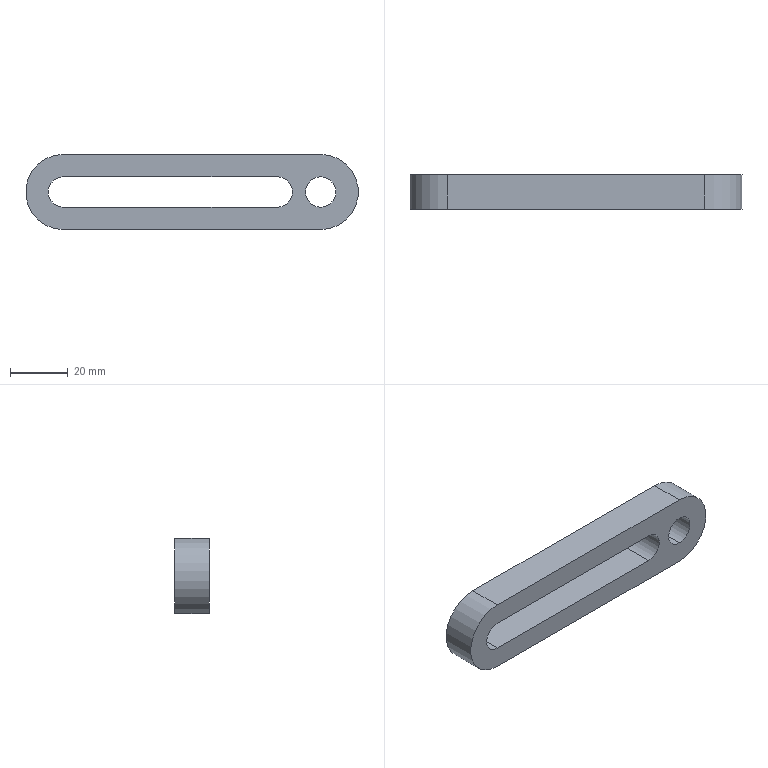Part | SolidWorks | features Extrusion 1 | 1 solid | 12 faces | box 115 x 12 x 26 mm | volume 22737 mm3 | cylinder 6 | plane 6 | commonest cylinder face diameters 10.5 x4 26 x2
STEP:
#1=CARTESIAN_POINT('',(44.5,6.,-5.25));
#2=VERTEX_POINT('',#1);
#3=CARTESIAN_POINT('',(44.5,6.,5.25));
#4=VERTEX_POINT('',#3);
#5=CARTESIAN_POINT('',(44.5,6.,0.));
#6=DIRECTION('',(0.,1.,0.));
#7=DIRECTION('',(0.,0.,1.));
#8=AXIS2_PLACEMENT_3D('',#5,#6,#7);
#9=CIRCLE('',#8,5.25);
#10=EDGE_CURVE('',#2,#4,#9,.T.);
#11=ORIENTED_EDGE('',*,*,#10,.T.);
#12=CARTESIAN_POINT('',(44.5,-6.,5.25));
#13=VERTEX_POINT('',#12);
#14=CARTESIAN_POINT('',(44.5,6.,5.25));
#15=DIRECTION('',(0.,-1.,0.));
#16=VECTOR('',#15,1000.);
#17=LINE('',#14,#16);
#18=EDGE_CURVE('',#4,#13,#17,.T.);
#19=ORIENTED_EDGE('',*,*,#18,.T.);
#20=CARTESIAN_POINT('',(44.5,-6.,-5.25));
#21=VERTEX_POINT('',#20);
#22=CARTESIAN_POINT('',(44.5,-6.,0.));
#23=DIRECTION('',(0.,1.,0.));
#24=DIRECTION('',(0.,0.,1.));
#25=AXIS2_PLACEMENT_3D('',#22,#23,#24);
#26=CIRCLE('',#25,5.25);
#27=EDGE_CURVE('',#21,#13,#26,.T.);
#28=ORIENTED_EDGE('',*,*,#27,.F.);
#29=CARTESIAN_POINT('',(44.5,6.,-5.25));
#30=DIRECTION('',(0.,-1.,0.));
#31=VECTOR('',#30,1000.);
#32=LINE('',#29,#31);
#33=EDGE_CURVE('',#2,#21,#32,.T.);
#34=ORIENTED_EDGE('',*,*,#33,.F.);
#35=EDGE_LOOP('',(#11,#19,#28,#34));
#36=FACE_OUTER_BOUND('',#35,.T.);
#37=CARTESIAN_POINT('',(44.5,6.,0.));
#38=DIRECTION('',(0.,-1.,0.));
#39=DIRECTION('',(0.,0.,-1.));
#40=AXIS2_PLACEMENT_3D('',#37,#38,#39);
#41=CYLINDRICAL_SURFACE('',#40,5.25);
#42=ADVANCED_FACE('',(#36),#41,.F.);
#43=CARTESIAN_POINT('',(-44.5,6.,5.25));
#44=VERTEX_POINT('',#43);
#45=CARTESIAN_POINT('',(29.5,6.,5.25));
#46=VERTEX_POINT('',#45);
#47=CARTESIAN_POINT('',(-44.5,6.,5.25));
#48=DIRECTION('',(1.,0.,0.));
#49=VECTOR('',#48,1000.);
#50=LINE('',#47,#49);
#51=EDGE_CURVE('',#44,#46,#50,.T.);
#52=ORIENTED_EDGE('',*,*,#51,.F.);
#53=CARTESIAN_POINT('',(-44.5,6.,-5.25));
#54=VERTEX_POINT('',#53);
#55=CARTESIAN_POINT('',(-44.5,6.,0.));
#56=DIRECTION('',(0.,1.,0.));
#57=DIRECTION('',(0.,0.,1.));
#58=AXIS2_PLACEMENT_3D('',#55,#56,#57);
#59=CIRCLE('',#58,5.25);
#60=EDGE_CURVE('',#54,#44,#59,.T.);
#61=ORIENTED_EDGE('',*,*,#60,.F.);
#62=CARTESIAN_POINT('',(29.5,6.,-5.25));
#63=VERTEX_POINT('',#62);
#64=CARTESIAN_POINT('',(-44.5,6.,-5.25));
#65=DIRECTION('',(-1.,0.,0.));
#66=VECTOR('',#65,1000.);
#67=LINE('',#64,#66);
#68=EDGE_CURVE('',#63,#54,#67,.T.);
#69=ORIENTED_EDGE('',*,*,#68,.F.);
#70=CARTESIAN_POINT('',(29.5,6.,0.));
#71=DIRECTION('',(0.,1.,0.));
#72=DIRECTION('',(0.,0.,1.));
#73=AXIS2_PLACEMENT_3D('',#70,#71,#72);
#74=CIRCLE('',#73,5.25);
#75=EDGE_CURVE('',#46,#63,#74,.T.);
#76=ORIENTED_EDGE('',*,*,#75,.F.);
#77=EDGE_LOOP('',(#52,#61,#69,#76));
#78=FACE_BOUND('',#77,.T.);
#79=CARTESIAN_POINT('',(-44.5,6.,-13.));
#80=VERTEX_POINT('',#79);
#81=CARTESIAN_POINT('',(-44.5,6.,13.));
#82=VERTEX_POINT('',#81);
#83=CARTESIAN_POINT('',(-44.5,6.,0.));
#84=DIRECTION('',(0.,1.,0.));
#85=DIRECTION('',(0.,0.,1.));
#86=AXIS2_PLACEMENT_3D('',#83,#84,#85);
#87=CIRCLE('',#86,13.);
#88=EDGE_CURVE('',#80,#82,#87,.T.);
#89=ORIENTED_EDGE('',*,*,#88,.T.);
#90=CARTESIAN_POINT('',(44.5,6.,13.));
#91=VERTEX_POINT('',#90);
#92=CARTESIAN_POINT('',(-44.5,6.,13.));
#93=DIRECTION('',(1.,0.,0.));
#94=VECTOR('',#93,1000.);
#95=LINE('',#92,#94);
#96=EDGE_CURVE('',#82,#91,#95,.T.);
#97=ORIENTED_EDGE('',*,*,#96,.T.);
#98=CARTESIAN_POINT('',(44.5,6.,-13.));
#99=VERTEX_POINT('',#98);
#100=CARTESIAN_POINT('',(44.5,6.,0.));
#101=DIRECTION('',(0.,1.,0.));
#102=DIRECTION('',(0.,0.,1.));
#103=AXIS2_PLACEMENT_3D('',#100,#101,#102);
#104=CIRCLE('',#103,13.);
#105=EDGE_CURVE('',#91,#99,#104,.T.);
#106=ORIENTED_EDGE('',*,*,#105,.T.);
#107=CARTESIAN_POINT('',(-44.5,6.,-13.));
#108=DIRECTION('',(-1.,0.,0.));
#109=VECTOR('',#108,1000.);
#110=LINE('',#107,#109);
#111=EDGE_CURVE('',#99,#80,#110,.T.);
#112=ORIENTED_EDGE('',*,*,#111,.T.);
#113=EDGE_LOOP('',(#89,#97,#106,#112));
#114=FACE_OUTER_BOUND('',#113,.T.);
#115=ORIENTED_EDGE('',*,*,#10,.F.);
#116=CARTESIAN_POINT('',(44.5,6.,0.));
#117=DIRECTION('',(0.,1.,0.));
#118=DIRECTION('',(0.,0.,1.));
#119=AXIS2_PLACEMENT_3D('',#116,#117,#118);
#120=CIRCLE('',#119,5.25);
#121=EDGE_CURVE('',#4,#2,#120,.T.);
#122=ORIENTED_EDGE('',*,*,#121,.F.);
#123=EDGE_LOOP('',(#115,#122));
#124=FACE_BOUND('',#123,.T.);
#125=CARTESIAN_POINT('',(-44.5,6.,0.));
#126=DIRECTION('',(0.,1.,0.));
#127=DIRECTION('',(0.,0.,1.));
#128=AXIS2_PLACEMENT_3D('',#125,#126,#127);
#129=PLANE('',#128);
#130=ADVANCED_FACE('',(#78,#114,#124),#129,.T.);
#131=CARTESIAN_POINT('',(-44.5,-6.,-5.25));
#132=VERTEX_POINT('',#131);
#133=CARTESIAN_POINT('',(-44.5,-6.,5.25));
#134=VERTEX_POINT('',#133);
#135=CARTESIAN_POINT('',(-44.5,-6.,0.));
#136=DIRECTION('',(0.,1.,0.));
#137=DIRECTION('',(0.,0.,1.));
#138=AXIS2_PLACEMENT_3D('',#135,#136,#137);
#139=CIRCLE('',#138,5.25);
#140=EDGE_CURVE('',#132,#134,#139,.T.);
#141=ORIENTED_EDGE('',*,*,#140,.T.);
#142=CARTESIAN_POINT('',(29.5,-6.,5.25));
#143=VERTEX_POINT('',#142);
#144=CARTESIAN_POINT('',(-44.5,-6.,5.25));
#145=DIRECTION('',(1.,0.,0.));
#146=VECTOR('',#145,1000.);
#147=LINE('',#144,#146);
#148=EDGE_CURVE('',#134,#143,#147,.T.);
#149=ORIENTED_EDGE('',*,*,#148,.T.);
#150=CARTESIAN_POINT('',(29.5,-6.,-5.25));
#151=VERTEX_POINT('',#150);
#152=CARTESIAN_POINT('',(29.5,-6.,0.));
#153=DIRECTION('',(0.,1.,0.));
#154=DIRECTION('',(0.,0.,1.));
#155=AXIS2_PLACEMENT_3D('',#152,#153,#154);
#156=CIRCLE('',#155,5.25);
#157=EDGE_CURVE('',#143,#151,#156,.T.);
#158=ORIENTED_EDGE('',*,*,#157,.T.);
#159=CARTESIAN_POINT('',(-44.5,-6.,-5.25));
#160=DIRECTION('',(-1.,0.,0.));
#161=VECTOR('',#160,1000.);
#162=LINE('',#159,#161);
#163=EDGE_CURVE('',#151,#132,#162,.T.);
#164=ORIENTED_EDGE('',*,*,#163,.T.);
#165=EDGE_LOOP('',(#141,#149,#158,#164));
#166=FACE_BOUND('',#165,.T.);
#167=CARTESIAN_POINT('',(-44.5,-6.,-13.));
#168=VERTEX_POINT('',#167);
#169=CARTESIAN_POINT('',(-44.5,-6.,13.));
#170=VERTEX_POINT('',#169);
#171=CARTESIAN_POINT('',(-44.5,-6.,0.));
#172=DIRECTION('',(0.,1.,0.));
#173=DIRECTION('',(0.,0.,1.));
#174=AXIS2_PLACEMENT_3D('',#171,#172,#173);
#175=CIRCLE('',#174,13.);
#176=EDGE_CURVE('',#168,#170,#175,.T.);
#177=ORIENTED_EDGE('',*,*,#176,.F.);
#178=CARTESIAN_POINT('',(44.5,-6.,-13.));
#179=VERTEX_POINT('',#178);
#180=CARTESIAN_POINT('',(-44.5,-6.,-13.));
#181=DIRECTION('',(-1.,0.,0.));
#182=VECTOR('',#181,1000.);
#183=LINE('',#180,#182);
#184=EDGE_CURVE('',#179,#168,#183,.T.);
#185=ORIENTED_EDGE('',*,*,#184,.F.);
#186=CARTESIAN_POINT('',(44.5,-6.,13.));
#187=VERTEX_POINT('',#186);
#188=CARTESIAN_POINT('',(44.5,-6.,0.));
#189=DIRECTION('',(0.,1.,0.));
#190=DIRECTION('',(0.,0.,1.));
#191=AXIS2_PLACEMENT_3D('',#188,#189,#190);
#192=CIRCLE('',#191,13.);
#193=EDGE_CURVE('',#187,#179,#192,.T.);
#194=ORIENTED_EDGE('',*,*,#193,.F.);
#195=CARTESIAN_POINT('',(-44.5,-6.,13.));
#196=DIRECTION('',(1.,0.,0.));
#197=VECTOR('',#196,1000.);
#198=LINE('',#195,#197);
#199=EDGE_CURVE('',#170,#187,#198,.T.);
#200=ORIENTED_EDGE('',*,*,#199,.F.);
#201=EDGE_LOOP('',(#177,#185,#194,#200));
#202=FACE_OUTER_BOUND('',#201,.T.);
#203=ORIENTED_EDGE('',*,*,#27,.T.);
#204=CARTESIAN_POINT('',(44.5,-6.,0.));
#205=DIRECTION('',(0.,1.,0.));
#206=DIRECTION('',(0.,0.,1.));
#207=AXIS2_PLACEMENT_3D('',#204,#205,#206);
#208=CIRCLE('',#207,5.25);
#209=EDGE_CURVE('',#13,#21,#208,.T.);
#210=ORIENTED_EDGE('',*,*,#209,.T.);
#211=EDGE_LOOP('',(#203,#210));
#212=FACE_BOUND('',#211,.T.);
#213=CARTESIAN_POINT('',(-44.5,-6.,0.));
#214=DIRECTION('',(0.,1.,0.));
#215=DIRECTION('',(0.,0.,1.));
#216=AXIS2_PLACEMENT_3D('',#213,#214,#215);
#217=PLANE('',#216);
#218=ADVANCED_FACE('',(#166,#202,#212),#217,.F.);
#219=ORIENTED_EDGE('',*,*,#176,.T.);
#220=CARTESIAN_POINT('',(-44.5,6.,13.));
#221=DIRECTION('',(0.,-1.,0.));
#222=VECTOR('',#221,1000.);
#223=LINE('',#220,#222);
#224=EDGE_CURVE('',#82,#170,#223,.T.);
#225=ORIENTED_EDGE('',*,*,#224,.F.);
#226=ORIENTED_EDGE('',*,*,#88,.F.);
#227=CARTESIAN_POINT('',(-44.5,6.,-13.));
#228=DIRECTION('',(0.,-1.,0.));
#229=VECTOR('',#228,1000.);
#230=LINE('',#227,#229);
#231=EDGE_CURVE('',#80,#168,#230,.T.);
#232=ORIENTED_EDGE('',*,*,#231,.T.);
#233=EDGE_LOOP('',(#219,#225,#226,#232));
#234=FACE_OUTER_BOUND('',#233,.T.);
#235=CARTESIAN_POINT('',(-44.5,6.,0.));
#236=DIRECTION('',(0.,-1.,0.));
#237=DIRECTION('',(0.,0.,-1.));
#238=AXIS2_PLACEMENT_3D('',#235,#236,#237);
#239=CYLINDRICAL_SURFACE('',#238,13.);
#240=ADVANCED_FACE('',(#234),#239,.T.);
#241=ORIENTED_EDGE('',*,*,#199,.T.);
#242=CARTESIAN_POINT('',(44.5,6.,13.));
#243=DIRECTION('',(0.,-1.,0.));
#244=VECTOR('',#243,1000.);
#245=LINE('',#242,#244);
#246=EDGE_CURVE('',#91,#187,#245,.T.);
#247=ORIENTED_EDGE('',*,*,#246,.F.);
#248=ORIENTED_EDGE('',*,*,#96,.F.);
#249=ORIENTED_EDGE('',*,*,#224,.T.);
#250=EDGE_LOOP('',(#241,#247,#248,#249));
#251=FACE_OUTER_BOUND('',#250,.T.);
#252=CARTESIAN_POINT('',(-44.5,6.,13.));
#253=DIRECTION('',(0.,0.,-1.));
#254=DIRECTION('',(-1.,0.,0.));
#255=AXIS2_PLACEMENT_3D('',#252,#253,#254);
#256=PLANE('',#255);
#257=ADVANCED_FACE('',(#251),#256,.F.);
#258=ORIENTED_EDGE('',*,*,#193,.T.);
#259=CARTESIAN_POINT('',(44.5,6.,-13.));
#260=DIRECTION('',(0.,-1.,0.));
#261=VECTOR('',#260,1000.);
#262=LINE('',#259,#261);
#263=EDGE_CURVE('',#99,#179,#262,.T.);
#264=ORIENTED_EDGE('',*,*,#263,.F.);
#265=ORIENTED_EDGE('',*,*,#105,.F.);
#266=ORIENTED_EDGE('',*,*,#246,.T.);
#267=EDGE_LOOP('',(#258,#264,#265,#266));
#268=FACE_OUTER_BOUND('',#267,.T.);
#269=CARTESIAN_POINT('',(44.5,6.,0.));
#270=DIRECTION('',(0.,-1.,0.));
#271=DIRECTION('',(0.,0.,-1.));
#272=AXIS2_PLACEMENT_3D('',#269,#270,#271);
#273=CYLINDRICAL_SURFACE('',#272,13.);
#274=ADVANCED_FACE('',(#268),#273,.T.);
#275=ORIENTED_EDGE('',*,*,#184,.T.);
#276=ORIENTED_EDGE('',*,*,#231,.F.);
#277=ORIENTED_EDGE('',*,*,#111,.F.);
#278=ORIENTED_EDGE('',*,*,#263,.T.);
#279=EDGE_LOOP('',(#275,#276,#277,#278));
#280=FACE_OUTER_BOUND('',#279,.T.);
#281=CARTESIAN_POINT('',(-44.5,6.,-13.));
#282=DIRECTION('',(0.,0.,1.));
#283=DIRECTION('',(1.,0.,0.));
#284=AXIS2_PLACEMENT_3D('',#281,#282,#283);
#285=PLANE('',#284);
#286=ADVANCED_FACE('',(#280),#285,.F.);
#287=ORIENTED_EDGE('',*,*,#140,.F.);
#288=CARTESIAN_POINT('',(-44.5,6.,-5.25));
#289=DIRECTION('',(0.,-1.,0.));
#290=VECTOR('',#289,1000.);
#291=LINE('',#288,#290);
#292=EDGE_CURVE('',#54,#132,#291,.T.);
#293=ORIENTED_EDGE('',*,*,#292,.F.);
#294=ORIENTED_EDGE('',*,*,#60,.T.);
#295=CARTESIAN_POINT('',(-44.5,6.,5.25));
#296=DIRECTION('',(0.,-1.,0.));
#297=VECTOR('',#296,1000.);
#298=LINE('',#295,#297);
#299=EDGE_CURVE('',#44,#134,#298,.T.);
#300=ORIENTED_EDGE('',*,*,#299,.T.);
#301=EDGE_LOOP('',(#287,#293,#294,#300));
#302=FACE_OUTER_BOUND('',#301,.T.);
#303=CARTESIAN_POINT('',(-44.5,6.,0.));
#304=DIRECTION('',(0.,-1.,0.));
#305=DIRECTION('',(0.,0.,-1.));
#306=AXIS2_PLACEMENT_3D('',#303,#304,#305);
#307=CYLINDRICAL_SURFACE('',#306,5.25);
#308=ADVANCED_FACE('',(#302),#307,.F.);
#309=ORIENTED_EDGE('',*,*,#148,.F.);
#310=ORIENTED_EDGE('',*,*,#299,.F.);
#311=ORIENTED_EDGE('',*,*,#51,.T.);
#312=CARTESIAN_POINT('',(29.5,6.,5.25));
#313=DIRECTION('',(0.,-1.,0.));
#314=VECTOR('',#313,1000.);
#315=LINE('',#312,#314);
#316=EDGE_CURVE('',#46,#143,#315,.T.);
#317=ORIENTED_EDGE('',*,*,#316,.T.);
#318=EDGE_LOOP('',(#309,#310,#311,#317));
#319=FACE_OUTER_BOUND('',#318,.T.);
#320=CARTESIAN_POINT('',(-44.5,6.,5.25));
#321=DIRECTION('',(0.,0.,-1.));
#322=DIRECTION('',(-1.,0.,0.));
#323=AXIS2_PLACEMENT_3D('',#320,#321,#322);
#324=PLANE('',#323);
#325=ADVANCED_FACE('',(#319),#324,.T.);
#326=ORIENTED_EDGE('',*,*,#157,.F.);
#327=ORIENTED_EDGE('',*,*,#316,.F.);
#328=ORIENTED_EDGE('',*,*,#75,.T.);
#329=CARTESIAN_POINT('',(29.5,6.,-5.25));
#330=DIRECTION('',(0.,-1.,0.));
#331=VECTOR('',#330,1000.);
#332=LINE('',#329,#331);
#333=EDGE_CURVE('',#63,#151,#332,.T.);
#334=ORIENTED_EDGE('',*,*,#333,.T.);
#335=EDGE_LOOP('',(#326,#327,#328,#334));
#336=FACE_OUTER_BOUND('',#335,.T.);
#337=CARTESIAN_POINT('',(29.5,6.,0.));
#338=DIRECTION('',(0.,-1.,0.));
#339=DIRECTION('',(0.,0.,-1.));
#340=AXIS2_PLACEMENT_3D('',#337,#338,#339);
#341=CYLINDRICAL_SURFACE('',#340,5.25);
#342=ADVANCED_FACE('',(#336),#341,.F.);
#343=ORIENTED_EDGE('',*,*,#163,.F.);
#344=ORIENTED_EDGE('',*,*,#333,.F.);
#345=ORIENTED_EDGE('',*,*,#68,.T.);
#346=ORIENTED_EDGE('',*,*,#292,.T.);
#347=EDGE_LOOP('',(#343,#344,#345,#346));
#348=FACE_OUTER_BOUND('',#347,.T.);
#349=CARTESIAN_POINT('',(-44.5,6.,-5.25));
#350=DIRECTION('',(0.,0.,1.));
#351=DIRECTION('',(1.,0.,0.));
#352=AXIS2_PLACEMENT_3D('',#349,#350,#351);
#353=PLANE('',#352);
#354=ADVANCED_FACE('',(#348),#353,.T.);
#355=ORIENTED_EDGE('',*,*,#18,.F.);
#356=ORIENTED_EDGE('',*,*,#121,.T.);
#357=ORIENTED_EDGE('',*,*,#33,.T.);
#358=ORIENTED_EDGE('',*,*,#209,.F.);
#359=EDGE_LOOP('',(#355,#356,#357,#358));
#360=FACE_OUTER_BOUND('',#359,.T.);
#361=CARTESIAN_POINT('',(44.5,6.,0.));
#362=DIRECTION('',(0.,-1.,0.));
#363=DIRECTION('',(0.,0.,-1.));
#364=AXIS2_PLACEMENT_3D('',#361,#362,#363);
#365=CYLINDRICAL_SURFACE('',#364,5.25);
#366=ADVANCED_FACE('',(#360),#365,.F.);
#367=CLOSED_SHELL('',(#42,#130,#218,#240,#257,#274,#286,#308,#325,#342,#354,#366));
#368=MANIFOLD_SOLID_BREP('',#367);
#369=CARTESIAN_POINT('',(0.,0.,0.));
#370=DIRECTION('',(0.,0.,1.));
#371=DIRECTION('',(1.,0.,0.));
#372=AXIS2_PLACEMENT_3D('',#369,#370,#371);
#373=(LENGTH_UNIT()NAMED_UNIT(*)SI_UNIT(.MILLI.,.METRE.));
#374=UNCERTAINTY_MEASURE_WITH_UNIT(LENGTH_MEASURE(0.00001),#373,'','');
#375=(NAMED_UNIT(*)PLANE_ANGLE_UNIT()SI_UNIT($,.RADIAN.));
#376=(NAMED_UNIT(*)SI_UNIT($,.STERADIAN.)SOLID_ANGLE_UNIT());
#377=(GEOMETRIC_REPRESENTATION_CONTEXT(3)GLOBAL_UNCERTAINTY_ASSIGNED_CONTEXT((#374))GLOBAL_UNIT_ASSIGNED_CONTEXT((#373,#375,#376))REPRESENTATION_CONTEXT('',''));
#378=ADVANCED_BREP_SHAPE_REPRESENTATION('',(#368,#372),#377);